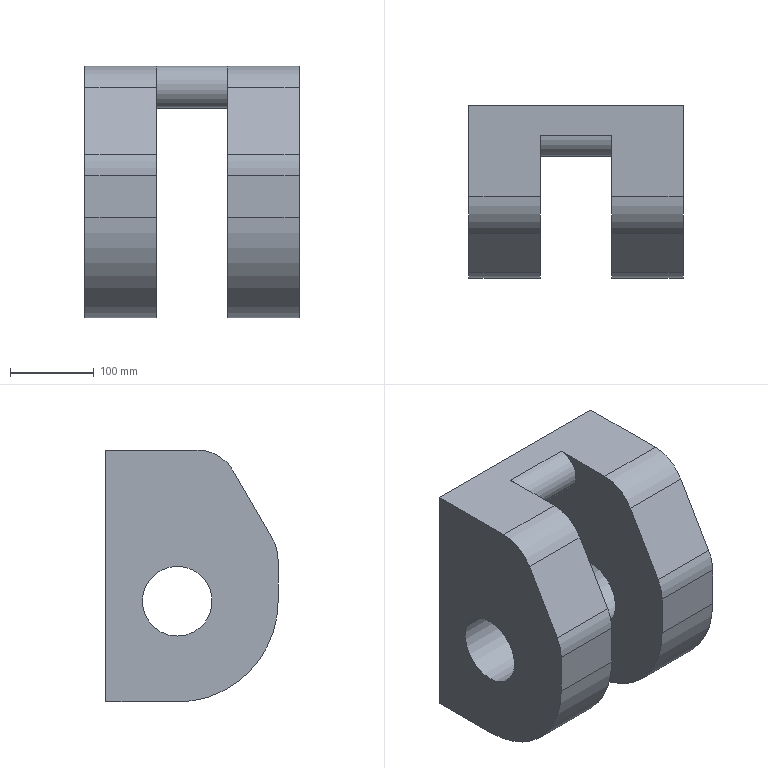Part | NX | features solid 2 | 1 solid | 22 faces | box 255 x 205 x 300 mm | volume 8542229 mm3 | plane 13 | cylinder 9 | commonest cylinder face diameters 100 x4 83 x2 240 x2 50 x1
STEP:
#1=CARTESIAN_POINT('',(-1395.,-1008.453,380.));
#2=VERTEX_POINT('',#1);
#3=CARTESIAN_POINT('',(-1395.,-935.,380.));
#4=VERTEX_POINT('',#3);
#5=CARTESIAN_POINT('',(-1395.,-1105.,380.));
#6=DIRECTION('',(0.,1.,0.));
#7=VECTOR('',#6,1000.);
#8=LINE('',#5,#7);
#9=EDGE_CURVE('',#2,#4,#8,.T.);
#10=ORIENTED_EDGE('',*,*,#9,.F.);
#11=CARTESIAN_POINT('',(-1310.,-1008.453,380.));
#12=VERTEX_POINT('',#11);
#13=CARTESIAN_POINT('',(-1310.,-1008.453,380.));
#14=DIRECTION('',(1.,0.,0.));
#15=VECTOR('',#14,1000.);
#16=LINE('',#13,#15);
#17=EDGE_CURVE('',#2,#12,#16,.T.);
#18=ORIENTED_EDGE('',*,*,#17,.T.);
#19=CARTESIAN_POINT('',(-1310.,-900.,380.));
#20=VERTEX_POINT('',#19);
#21=CARTESIAN_POINT('',(-1310.,-1105.,380.));
#22=DIRECTION('',(0.,1.,0.));
#23=VECTOR('',#22,1000.);
#24=LINE('',#21,#23);
#25=EDGE_CURVE('',#12,#20,#24,.T.);
#26=ORIENTED_EDGE('',*,*,#25,.T.);
#27=CARTESIAN_POINT('',(-1565.,-900.,380.));
#28=VERTEX_POINT('',#27);
#29=CARTESIAN_POINT('',(-1565.,-900.,380.));
#30=DIRECTION('',(1.,0.,0.));
#31=VECTOR('',#30,1000.);
#32=LINE('',#29,#31);
#33=EDGE_CURVE('',#28,#20,#32,.T.);
#34=ORIENTED_EDGE('',*,*,#33,.F.);
#35=CARTESIAN_POINT('',(-1565.,-1008.453,380.));
#36=VERTEX_POINT('',#35);
#37=CARTESIAN_POINT('',(-1565.,-1105.,380.));
#38=DIRECTION('',(0.,1.,0.));
#39=VECTOR('',#38,1000.);
#40=LINE('',#37,#39);
#41=EDGE_CURVE('',#36,#28,#40,.T.);
#42=ORIENTED_EDGE('',*,*,#41,.F.);
#43=CARTESIAN_POINT('',(-1480.,-1008.453,380.));
#44=VERTEX_POINT('',#43);
#45=CARTESIAN_POINT('',(-1480.,-1008.453,380.));
#46=DIRECTION('',(1.,0.,0.));
#47=VECTOR('',#46,1000.);
#48=LINE('',#45,#47);
#49=EDGE_CURVE('',#36,#44,#48,.T.);
#50=ORIENTED_EDGE('',*,*,#49,.T.);
#51=CARTESIAN_POINT('',(-1480.,-935.,380.));
#52=VERTEX_POINT('',#51);
#53=CARTESIAN_POINT('',(-1480.,-1105.,380.));
#54=DIRECTION('',(0.,1.,0.));
#55=VECTOR('',#54,1000.);
#56=LINE('',#53,#55);
#57=EDGE_CURVE('',#44,#52,#56,.T.);
#58=ORIENTED_EDGE('',*,*,#57,.T.);
#59=CARTESIAN_POINT('',(-1437.5,-935.,380.));
#60=DIRECTION('',(1.,0.,0.));
#61=VECTOR('',#60,1000.);
#62=LINE('',#59,#61);
#63=EDGE_CURVE('',#4,#52,#62,.F.);
#64=ORIENTED_EDGE('',*,*,#63,.F.);
#65=EDGE_LOOP('',(#10,#18,#26,#34,#42,#50,#58,#64));
#66=FACE_BOUND('',#65,.T.);
#67=CARTESIAN_POINT('',(-1565.,-1105.,380.));
#68=DIRECTION('',(0.,0.,-1.));
#69=DIRECTION('',(0.,1.,0.));
#70=AXIS2_PLACEMENT_3D('',#67,#68,#69);
#71=PLANE('',#70);
#72=ADVANCED_FACE('',(#66),#71,.F.);
#73=CARTESIAN_POINT('',(-1565.,-985.,80.));
#74=VERTEX_POINT('',#73);
#75=CARTESIAN_POINT('',(-1565.,-900.,80.));
#76=VERTEX_POINT('',#75);
#77=CARTESIAN_POINT('',(-1565.,-1105.,80.));
#78=DIRECTION('',(0.,1.,0.));
#79=VECTOR('',#78,1000.);
#80=LINE('',#77,#79);
#81=EDGE_CURVE('',#74,#76,#80,.T.);
#82=ORIENTED_EDGE('',*,*,#81,.T.);
#83=CARTESIAN_POINT('',(-1480.,-900.,80.));
#84=VERTEX_POINT('',#83);
#85=CARTESIAN_POINT('',(-1565.,-900.,80.));
#86=DIRECTION('',(1.,0.,0.));
#87=VECTOR('',#86,1000.);
#88=LINE('',#85,#87);
#89=EDGE_CURVE('',#76,#84,#88,.T.);
#90=ORIENTED_EDGE('',*,*,#89,.T.);
#91=CARTESIAN_POINT('',(-1480.,-985.,80.));
#92=VERTEX_POINT('',#91);
#93=CARTESIAN_POINT('',(-1480.,-1105.,80.));
#94=DIRECTION('',(0.,-1.,0.));
#95=VECTOR('',#94,1000.);
#96=LINE('',#93,#95);
#97=EDGE_CURVE('',#92,#84,#96,.F.);
#98=ORIENTED_EDGE('',*,*,#97,.F.);
#99=CARTESIAN_POINT('',(-1565.,-985.,80.));
#100=DIRECTION('',(-1.,0.,0.));
#101=VECTOR('',#100,1000.);
#102=LINE('',#99,#101);
#103=EDGE_CURVE('',#74,#92,#102,.F.);
#104=ORIENTED_EDGE('',*,*,#103,.F.);
#105=EDGE_LOOP('',(#82,#90,#98,#104));
#106=FACE_BOUND('',#105,.T.);
#107=CARTESIAN_POINT('',(-1565.,-1105.,80.));
#108=DIRECTION('',(0.,0.,-1.));
#109=DIRECTION('',(0.,1.,0.));
#110=AXIS2_PLACEMENT_3D('',#107,#108,#109);
#111=PLANE('',#110);
#112=ADVANCED_FACE('',(#106),#111,.T.);
#113=CARTESIAN_POINT('',(-1480.,-1105.,200.));
#114=VERTEX_POINT('',#113);
#115=CARTESIAN_POINT('',(-1480.,-1105.,249.378));
#116=VERTEX_POINT('',#115);
#117=CARTESIAN_POINT('',(-1480.,-1105.,80.));
#118=DIRECTION('',(0.,0.,1.));
#119=VECTOR('',#118,1000.);
#120=LINE('',#117,#119);
#121=EDGE_CURVE('',#114,#116,#120,.T.);
#122=ORIENTED_EDGE('',*,*,#121,.T.);
#123=CARTESIAN_POINT('',(-1565.,-1105.,249.378));
#124=VERTEX_POINT('',#123);
#125=CARTESIAN_POINT('',(-1565.,-1105.,249.378));
#126=DIRECTION('',(-1.,0.,0.));
#127=VECTOR('',#126,1000.);
#128=LINE('',#125,#127);
#129=EDGE_CURVE('',#116,#124,#128,.T.);
#130=ORIENTED_EDGE('',*,*,#129,.T.);
#131=CARTESIAN_POINT('',(-1565.,-1105.,200.));
#132=VERTEX_POINT('',#131);
#133=CARTESIAN_POINT('',(-1565.,-1105.,80.));
#134=DIRECTION('',(0.,0.,1.));
#135=VECTOR('',#134,1000.);
#136=LINE('',#133,#135);
#137=EDGE_CURVE('',#132,#124,#136,.T.);
#138=ORIENTED_EDGE('',*,*,#137,.F.);
#139=CARTESIAN_POINT('',(-1565.,-1105.,200.));
#140=DIRECTION('',(1.,0.,0.));
#141=VECTOR('',#140,1000.);
#142=LINE('',#139,#141);
#143=EDGE_CURVE('',#114,#132,#142,.F.);
#144=ORIENTED_EDGE('',*,*,#143,.F.);
#145=EDGE_LOOP('',(#122,#130,#138,#144));
#146=FACE_BOUND('',#145,.T.);
#147=CARTESIAN_POINT('',(-1565.,-1105.,80.));
#148=DIRECTION('',(0.,1.,0.));
#149=DIRECTION('',(0.,0.,1.));
#150=AXIS2_PLACEMENT_3D('',#147,#148,#149);
#151=PLANE('',#150);
#152=ADVANCED_FACE('',(#146),#151,.F.);
#153=CARTESIAN_POINT('',(-1310.,-900.,80.));
#154=VERTEX_POINT('',#153);
#155=CARTESIAN_POINT('',(-1310.,-900.,45.));
#156=DIRECTION('',(0.,0.,1.));
#157=VECTOR('',#156,1000.);
#158=LINE('',#155,#157);
#159=EDGE_CURVE('',#154,#20,#158,.T.);
#160=ORIENTED_EDGE('',*,*,#159,.F.);
#161=CARTESIAN_POINT('',(-1395.,-900.,80.));
#162=VERTEX_POINT('',#161);
#163=CARTESIAN_POINT('',(-1395.,-900.,80.));
#164=DIRECTION('',(1.,0.,0.));
#165=VECTOR('',#164,1000.);
#166=LINE('',#163,#165);
#167=EDGE_CURVE('',#162,#154,#166,.T.);
#168=ORIENTED_EDGE('',*,*,#167,.F.);
#169=CARTESIAN_POINT('',(-1395.,-900.,330.));
#170=VERTEX_POINT('',#169);
#171=CARTESIAN_POINT('',(-1395.,-900.,45.));
#172=DIRECTION('',(0.,0.,1.));
#173=VECTOR('',#172,1000.);
#174=LINE('',#171,#173);
#175=EDGE_CURVE('',#162,#170,#174,.T.);
#176=ORIENTED_EDGE('',*,*,#175,.T.);
#177=CARTESIAN_POINT('',(-1480.,-900.,330.));
#178=VERTEX_POINT('',#177);
#179=CARTESIAN_POINT('',(-1437.5,-900.,330.));
#180=DIRECTION('',(1.,0.,0.));
#181=VECTOR('',#180,1000.);
#182=LINE('',#179,#181);
#183=EDGE_CURVE('',#178,#170,#182,.T.);
#184=ORIENTED_EDGE('',*,*,#183,.F.);
#185=CARTESIAN_POINT('',(-1480.,-900.,45.));
#186=DIRECTION('',(0.,0.,1.));
#187=VECTOR('',#186,1000.);
#188=LINE('',#185,#187);
#189=EDGE_CURVE('',#84,#178,#188,.T.);
#190=ORIENTED_EDGE('',*,*,#189,.F.);
#191=ORIENTED_EDGE('',*,*,#89,.F.);
#192=CARTESIAN_POINT('',(-1565.,-900.,45.));
#193=DIRECTION('',(0.,0.,1.));
#194=VECTOR('',#193,1000.);
#195=LINE('',#192,#194);
#196=EDGE_CURVE('',#76,#28,#195,.T.);
#197=ORIENTED_EDGE('',*,*,#196,.T.);
#198=ORIENTED_EDGE('',*,*,#33,.T.);
#199=EDGE_LOOP('',(#160,#168,#176,#184,#190,#191,#197,#198));
#200=FACE_BOUND('',#199,.T.);
#201=CARTESIAN_POINT('',(-1565.,-900.,45.));
#202=DIRECTION('',(0.,1.,0.));
#203=DIRECTION('',(0.,0.,1.));
#204=AXIS2_PLACEMENT_3D('',#201,#202,#203);
#205=PLANE('',#204);
#206=ADVANCED_FACE('',(#200),#205,.T.);
#207=ORIENTED_EDGE('',*,*,#57,.F.);
#208=CARTESIAN_POINT('',(-1480.,-1051.754,355.));
#209=VERTEX_POINT('',#208);
#210=CARTESIAN_POINT('',(-1480.,-1008.453,330.));
#211=DIRECTION('',(-1.,0.,0.));
#212=DIRECTION('',(0.,0.,-1.));
#213=AXIS2_PLACEMENT_3D('',#210,#211,#212);
#214=CIRCLE('',#213,50.);
#215=EDGE_CURVE('',#44,#209,#214,.F.);
#216=ORIENTED_EDGE('',*,*,#215,.T.);
#217=CARTESIAN_POINT('',(-1480.,-1098.301,274.378));
#218=VERTEX_POINT('',#217);
#219=CARTESIAN_POINT('',(-1480.,-1174.286,142.769));
#220=DIRECTION('',(0.,0.5,0.866));
#221=VECTOR('',#220,1000.);
#222=LINE('',#219,#221);
#223=EDGE_CURVE('',#218,#209,#222,.T.);
#224=ORIENTED_EDGE('',*,*,#223,.F.);
#225=CARTESIAN_POINT('',(-1480.,-1055.,249.378));
#226=DIRECTION('',(-1.,0.,0.));
#227=DIRECTION('',(0.,0.,-1.));
#228=AXIS2_PLACEMENT_3D('',#225,#226,#227);
#229=CIRCLE('',#228,50.);
#230=EDGE_CURVE('',#218,#116,#229,.F.);
#231=ORIENTED_EDGE('',*,*,#230,.T.);
#232=ORIENTED_EDGE('',*,*,#121,.F.);
#233=CARTESIAN_POINT('',(-1480.,-985.,200.));
#234=DIRECTION('',(1.,0.,0.));
#235=DIRECTION('',(0.,0.,1.));
#236=AXIS2_PLACEMENT_3D('',#233,#234,#235);
#237=CIRCLE('',#236,120.);
#238=EDGE_CURVE('',#92,#114,#237,.F.);
#239=ORIENTED_EDGE('',*,*,#238,.F.);
#240=ORIENTED_EDGE('',*,*,#97,.T.);
#241=ORIENTED_EDGE('',*,*,#189,.T.);
#242=CARTESIAN_POINT('',(-1480.,-935.,330.));
#243=VERTEX_POINT('',#242);
#244=CARTESIAN_POINT('',(-1480.,-930.,330.));
#245=DIRECTION('',(0.,1.,0.));
#246=VECTOR('',#245,1000.);
#247=LINE('',#244,#246);
#248=EDGE_CURVE('',#243,#178,#247,.T.);
#249=ORIENTED_EDGE('',*,*,#248,.F.);
#250=CARTESIAN_POINT('',(-1480.,-935.,355.));
#251=DIRECTION('',(1.,0.,0.));
#252=DIRECTION('',(0.,0.,1.));
#253=AXIS2_PLACEMENT_3D('',#250,#251,#252);
#254=CIRCLE('',#253,25.);
#255=EDGE_CURVE('',#52,#243,#254,.T.);
#256=ORIENTED_EDGE('',*,*,#255,.F.);
#257=EDGE_LOOP('',(#207,#216,#224,#231,#232,#239,#240,#241,#249,#256));
#258=FACE_BOUND('',#257,.T.);
#259=CARTESIAN_POINT('',(-1480.,-985.,241.5));
#260=VERTEX_POINT('',#259);
#261=CARTESIAN_POINT('',(-1480.,-985.,200.));
#262=DIRECTION('',(1.,0.,0.));
#263=DIRECTION('',(0.,0.,1.));
#264=AXIS2_PLACEMENT_3D('',#261,#262,#263);
#265=CIRCLE('',#264,41.5);
#266=EDGE_CURVE('',#260,#260,#265,.T.);
#267=ORIENTED_EDGE('',*,*,#266,.F.);
#268=EDGE_LOOP('',(#267));
#269=FACE_BOUND('',#268,.T.);
#270=CARTESIAN_POINT('',(-1480.,-1105.,45.));
#271=DIRECTION('',(-1.,0.,0.));
#272=DIRECTION('',(0.,0.,1.));
#273=AXIS2_PLACEMENT_3D('',#270,#271,#272);
#274=PLANE('',#273);
#275=ADVANCED_FACE('',(#258,#269),#274,.F.);
#276=CARTESIAN_POINT('',(-1565.,-1098.301,274.378));
#277=VERTEX_POINT('',#276);
#278=CARTESIAN_POINT('',(-1565.,-1051.754,355.));
#279=VERTEX_POINT('',#278);
#280=CARTESIAN_POINT('',(-1565.,-1174.286,142.769));
#281=DIRECTION('',(0.,0.5,0.866));
#282=VECTOR('',#281,1000.);
#283=LINE('',#280,#282);
#284=EDGE_CURVE('',#277,#279,#283,.T.);
#285=ORIENTED_EDGE('',*,*,#284,.T.);
#286=CARTESIAN_POINT('',(-1565.,-1008.453,330.));
#287=DIRECTION('',(-1.,0.,0.));
#288=DIRECTION('',(0.,0.,-1.));
#289=AXIS2_PLACEMENT_3D('',#286,#287,#288);
#290=CIRCLE('',#289,50.);
#291=EDGE_CURVE('',#279,#36,#290,.T.);
#292=ORIENTED_EDGE('',*,*,#291,.T.);
#293=ORIENTED_EDGE('',*,*,#41,.T.);
#294=ORIENTED_EDGE('',*,*,#196,.F.);
#295=ORIENTED_EDGE('',*,*,#81,.F.);
#296=CARTESIAN_POINT('',(-1565.,-985.,200.));
#297=DIRECTION('',(1.,0.,0.));
#298=DIRECTION('',(0.,0.,1.));
#299=AXIS2_PLACEMENT_3D('',#296,#297,#298);
#300=CIRCLE('',#299,120.);
#301=EDGE_CURVE('',#132,#74,#300,.T.);
#302=ORIENTED_EDGE('',*,*,#301,.F.);
#303=ORIENTED_EDGE('',*,*,#137,.T.);
#304=CARTESIAN_POINT('',(-1565.,-1055.,249.378));
#305=DIRECTION('',(-1.,0.,0.));
#306=DIRECTION('',(0.,0.,-1.));
#307=AXIS2_PLACEMENT_3D('',#304,#305,#306);
#308=CIRCLE('',#307,50.);
#309=EDGE_CURVE('',#124,#277,#308,.T.);
#310=ORIENTED_EDGE('',*,*,#309,.T.);
#311=EDGE_LOOP('',(#285,#292,#293,#294,#295,#302,#303,#310));
#312=FACE_BOUND('',#311,.T.);
#313=CARTESIAN_POINT('',(-1565.,-985.,158.5));
#314=VERTEX_POINT('',#313);
#315=CARTESIAN_POINT('',(-1565.,-985.,200.));
#316=DIRECTION('',(-1.,0.,0.));
#317=DIRECTION('',(0.,0.,-1.));
#318=AXIS2_PLACEMENT_3D('',#315,#316,#317);
#319=CIRCLE('',#318,41.5);
#320=EDGE_CURVE('',#314,#314,#319,.T.);
#321=ORIENTED_EDGE('',*,*,#320,.F.);
#322=EDGE_LOOP('',(#321));
#323=FACE_BOUND('',#322,.T.);
#324=CARTESIAN_POINT('',(-1565.,-1105.,45.));
#325=DIRECTION('',(-1.,0.,0.));
#326=DIRECTION('',(0.,0.,1.));
#327=AXIS2_PLACEMENT_3D('',#324,#325,#326);
#328=PLANE('',#327);
#329=ADVANCED_FACE('',(#312,#323),#328,.T.);
#330=ORIENTED_EDGE('',*,*,#301,.T.);
#331=ORIENTED_EDGE('',*,*,#103,.T.);
#332=ORIENTED_EDGE('',*,*,#238,.T.);
#333=ORIENTED_EDGE('',*,*,#143,.T.);
#334=EDGE_LOOP('',(#330,#331,#332,#333));
#335=FACE_BOUND('',#334,.T.);
#336=CARTESIAN_POINT('',(-1565.,-985.,200.));
#337=DIRECTION('',(-1.,0.,0.));
#338=DIRECTION('',(0.,0.,1.));
#339=AXIS2_PLACEMENT_3D('',#336,#337,#338);
#340=CYLINDRICAL_SURFACE('',#339,120.);
#341=ADVANCED_FACE('',(#335),#340,.T.);
#342=ORIENTED_EDGE('',*,*,#320,.T.);
#343=EDGE_LOOP('',(#342));
#344=FACE_BOUND('',#343,.T.);
#345=ORIENTED_EDGE('',*,*,#266,.T.);
#346=EDGE_LOOP('',(#345));
#347=FACE_BOUND('',#346,.T.);
#348=CARTESIAN_POINT('',(-1565.,-985.,200.));
#349=DIRECTION('',(1.,0.,0.));
#350=DIRECTION('',(0.,0.,-1.));
#351=AXIS2_PLACEMENT_3D('',#348,#349,#350);
#352=CYLINDRICAL_SURFACE('',#351,41.5);
#353=ADVANCED_FACE('',(#344,#347),#352,.F.);
#354=ORIENTED_EDGE('',*,*,#248,.T.);
#355=ORIENTED_EDGE('',*,*,#183,.T.);
#356=CARTESIAN_POINT('',(-1395.,-935.,330.));
#357=VERTEX_POINT('',#356);
#358=CARTESIAN_POINT('',(-1395.,-930.,330.));
#359=DIRECTION('',(0.,-1.,0.));
#360=VECTOR('',#359,1000.);
#361=LINE('',#358,#360);
#362=EDGE_CURVE('',#170,#357,#361,.T.);
#363=ORIENTED_EDGE('',*,*,#362,.T.);
#364=CARTESIAN_POINT('',(-1437.5,-935.,330.));
#365=DIRECTION('',(-1.,0.,0.));
#366=VECTOR('',#365,1000.);
#367=LINE('',#364,#366);
#368=EDGE_CURVE('',#243,#357,#367,.F.);
#369=ORIENTED_EDGE('',*,*,#368,.F.);
#370=EDGE_LOOP('',(#354,#355,#363,#369));
#371=FACE_BOUND('',#370,.T.);
#372=CARTESIAN_POINT('',(-1437.5,-930.,330.));
#373=DIRECTION('',(0.,0.,-1.));
#374=DIRECTION('',(0.,-1.,0.));
#375=AXIS2_PLACEMENT_3D('',#372,#373,#374);
#376=PLANE('',#375);
#377=ADVANCED_FACE('',(#371),#376,.T.);
#378=ORIENTED_EDGE('',*,*,#368,.T.);
#379=CARTESIAN_POINT('',(-1395.,-935.,355.));
#380=DIRECTION('',(-1.,0.,0.));
#381=DIRECTION('',(0.,0.,-1.));
#382=AXIS2_PLACEMENT_3D('',#379,#380,#381);
#383=CIRCLE('',#382,25.);
#384=EDGE_CURVE('',#357,#4,#383,.T.);
#385=ORIENTED_EDGE('',*,*,#384,.T.);
#386=ORIENTED_EDGE('',*,*,#63,.T.);
#387=ORIENTED_EDGE('',*,*,#255,.T.);
#388=EDGE_LOOP('',(#378,#385,#386,#387));
#389=FACE_BOUND('',#388,.T.);
#390=CARTESIAN_POINT('',(-1437.5,-935.,355.));
#391=DIRECTION('',(-1.,0.,0.));
#392=DIRECTION('',(0.,0.,1.));
#393=AXIS2_PLACEMENT_3D('',#390,#391,#392);
#394=CYLINDRICAL_SURFACE('',#393,25.);
#395=ADVANCED_FACE('',(#389),#394,.T.);
#396=CARTESIAN_POINT('',(-1395.,-985.,80.));
#397=VERTEX_POINT('',#396);
#398=CARTESIAN_POINT('',(-1395.,-1105.,80.));
#399=DIRECTION('',(0.,1.,0.));
#400=VECTOR('',#399,1000.);
#401=LINE('',#398,#400);
#402=EDGE_CURVE('',#397,#162,#401,.T.);
#403=ORIENTED_EDGE('',*,*,#402,.T.);
#404=ORIENTED_EDGE('',*,*,#167,.T.);
#405=CARTESIAN_POINT('',(-1310.,-985.,80.));
#406=VERTEX_POINT('',#405);
#407=CARTESIAN_POINT('',(-1310.,-1105.,80.));
#408=DIRECTION('',(0.,-1.,0.));
#409=VECTOR('',#408,1000.);
#410=LINE('',#407,#409);
#411=EDGE_CURVE('',#406,#154,#410,.F.);
#412=ORIENTED_EDGE('',*,*,#411,.F.);
#413=CARTESIAN_POINT('',(-1395.,-985.,80.));
#414=DIRECTION('',(-1.,0.,0.));
#415=VECTOR('',#414,1000.);
#416=LINE('',#413,#415);
#417=EDGE_CURVE('',#397,#406,#416,.F.);
#418=ORIENTED_EDGE('',*,*,#417,.F.);
#419=EDGE_LOOP('',(#403,#404,#412,#418));
#420=FACE_BOUND('',#419,.T.);
#421=CARTESIAN_POINT('',(-1395.,-1105.,80.));
#422=DIRECTION('',(0.,0.,-1.));
#423=DIRECTION('',(0.,1.,0.));
#424=AXIS2_PLACEMENT_3D('',#421,#422,#423);
#425=PLANE('',#424);
#426=ADVANCED_FACE('',(#420),#425,.T.);
#427=CARTESIAN_POINT('',(-1310.,-1105.,200.));
#428=VERTEX_POINT('',#427);
#429=CARTESIAN_POINT('',(-1310.,-1105.,249.378));
#430=VERTEX_POINT('',#429);
#431=CARTESIAN_POINT('',(-1310.,-1105.,80.));
#432=DIRECTION('',(0.,0.,1.));
#433=VECTOR('',#432,1000.);
#434=LINE('',#431,#433);
#435=EDGE_CURVE('',#428,#430,#434,.T.);
#436=ORIENTED_EDGE('',*,*,#435,.T.);
#437=CARTESIAN_POINT('',(-1395.,-1105.,249.378));
#438=VERTEX_POINT('',#437);
#439=CARTESIAN_POINT('',(-1395.,-1105.,249.378));
#440=DIRECTION('',(-1.,0.,0.));
#441=VECTOR('',#440,1000.);
#442=LINE('',#439,#441);
#443=EDGE_CURVE('',#430,#438,#442,.T.);
#444=ORIENTED_EDGE('',*,*,#443,.T.);
#445=CARTESIAN_POINT('',(-1395.,-1105.,200.));
#446=VERTEX_POINT('',#445);
#447=CARTESIAN_POINT('',(-1395.,-1105.,80.));
#448=DIRECTION('',(0.,0.,1.));
#449=VECTOR('',#448,1000.);
#450=LINE('',#447,#449);
#451=EDGE_CURVE('',#446,#438,#450,.T.);
#452=ORIENTED_EDGE('',*,*,#451,.F.);
#453=CARTESIAN_POINT('',(-1395.,-1105.,200.));
#454=DIRECTION('',(1.,0.,0.));
#455=VECTOR('',#454,1000.);
#456=LINE('',#453,#455);
#457=EDGE_CURVE('',#428,#446,#456,.F.);
#458=ORIENTED_EDGE('',*,*,#457,.F.);
#459=EDGE_LOOP('',(#436,#444,#452,#458));
#460=FACE_BOUND('',#459,.T.);
#461=CARTESIAN_POINT('',(-1395.,-1105.,80.));
#462=DIRECTION('',(0.,1.,0.));
#463=DIRECTION('',(0.,0.,1.));
#464=AXIS2_PLACEMENT_3D('',#461,#462,#463);
#465=PLANE('',#464);
#466=ADVANCED_FACE('',(#460),#465,.F.);
#467=ORIENTED_EDGE('',*,*,#25,.F.);
#468=CARTESIAN_POINT('',(-1310.,-1051.754,355.));
#469=VERTEX_POINT('',#468);
#470=CARTESIAN_POINT('',(-1310.,-1008.453,330.));
#471=DIRECTION('',(-1.,0.,0.));
#472=DIRECTION('',(0.,0.,-1.));
#473=AXIS2_PLACEMENT_3D('',#470,#471,#472);
#474=CIRCLE('',#473,50.);
#475=EDGE_CURVE('',#12,#469,#474,.F.);
#476=ORIENTED_EDGE('',*,*,#475,.T.);
#477=CARTESIAN_POINT('',(-1310.,-1098.301,274.378));
#478=VERTEX_POINT('',#477);
#479=CARTESIAN_POINT('',(-1310.,-1174.286,142.769));
#480=DIRECTION('',(0.,0.5,0.866));
#481=VECTOR('',#480,1000.);
#482=LINE('',#479,#481);
#483=EDGE_CURVE('',#478,#469,#482,.T.);
#484=ORIENTED_EDGE('',*,*,#483,.F.);
#485=CARTESIAN_POINT('',(-1310.,-1055.,249.378));
#486=DIRECTION('',(-1.,0.,0.));
#487=DIRECTION('',(0.,0.,-1.));
#488=AXIS2_PLACEMENT_3D('',#485,#486,#487);
#489=CIRCLE('',#488,50.);
#490=EDGE_CURVE('',#478,#430,#489,.F.);
#491=ORIENTED_EDGE('',*,*,#490,.T.);
#492=ORIENTED_EDGE('',*,*,#435,.F.);
#493=CARTESIAN_POINT('',(-1310.,-985.,200.));
#494=DIRECTION('',(1.,0.,0.));
#495=DIRECTION('',(0.,0.,1.));
#496=AXIS2_PLACEMENT_3D('',#493,#494,#495);
#497=CIRCLE('',#496,120.);
#498=EDGE_CURVE('',#406,#428,#497,.F.);
#499=ORIENTED_EDGE('',*,*,#498,.F.);
#500=ORIENTED_EDGE('',*,*,#411,.T.);
#501=ORIENTED_EDGE('',*,*,#159,.T.);
#502=EDGE_LOOP('',(#467,#476,#484,#491,#492,#499,#500,#501));
#503=FACE_BOUND('',#502,.T.);
#504=CARTESIAN_POINT('',(-1310.,-985.,241.5));
#505=VERTEX_POINT('',#504);
#506=CARTESIAN_POINT('',(-1310.,-985.,200.));
#507=DIRECTION('',(1.,0.,0.));
#508=DIRECTION('',(0.,0.,1.));
#509=AXIS2_PLACEMENT_3D('',#506,#507,#508);
#510=CIRCLE('',#509,41.5);
#511=EDGE_CURVE('',#505,#505,#510,.T.);
#512=ORIENTED_EDGE('',*,*,#511,.F.);
#513=EDGE_LOOP('',(#512));
#514=FACE_BOUND('',#513,.T.);
#515=CARTESIAN_POINT('',(-1310.,-1105.,45.));
#516=DIRECTION('',(-1.,0.,0.));
#517=DIRECTION('',(0.,0.,1.));
#518=AXIS2_PLACEMENT_3D('',#515,#516,#517);
#519=PLANE('',#518);
#520=ADVANCED_FACE('',(#503,#514),#519,.F.);
#521=CARTESIAN_POINT('',(-1395.,-1098.301,274.378));
#522=VERTEX_POINT('',#521);
#523=CARTESIAN_POINT('',(-1395.,-1051.754,355.));
#524=VERTEX_POINT('',#523);
#525=CARTESIAN_POINT('',(-1395.,-1174.286,142.769));
#526=DIRECTION('',(0.,0.5,0.866));
#527=VECTOR('',#526,1000.);
#528=LINE('',#525,#527);
#529=EDGE_CURVE('',#522,#524,#528,.T.);
#530=ORIENTED_EDGE('',*,*,#529,.T.);
#531=CARTESIAN_POINT('',(-1395.,-1008.453,330.));
#532=DIRECTION('',(-1.,0.,0.));
#533=DIRECTION('',(0.,0.,-1.));
#534=AXIS2_PLACEMENT_3D('',#531,#532,#533);
#535=CIRCLE('',#534,50.);
#536=EDGE_CURVE('',#524,#2,#535,.T.);
#537=ORIENTED_EDGE('',*,*,#536,.T.);
#538=ORIENTED_EDGE('',*,*,#9,.T.);
#539=ORIENTED_EDGE('',*,*,#384,.F.);
#540=ORIENTED_EDGE('',*,*,#362,.F.);
#541=ORIENTED_EDGE('',*,*,#175,.F.);
#542=ORIENTED_EDGE('',*,*,#402,.F.);
#543=CARTESIAN_POINT('',(-1395.,-985.,200.));
#544=DIRECTION('',(1.,0.,0.));
#545=DIRECTION('',(0.,0.,1.));
#546=AXIS2_PLACEMENT_3D('',#543,#544,#545);
#547=CIRCLE('',#546,120.);
#548=EDGE_CURVE('',#446,#397,#547,.T.);
#549=ORIENTED_EDGE('',*,*,#548,.F.);
#550=ORIENTED_EDGE('',*,*,#451,.T.);
#551=CARTESIAN_POINT('',(-1395.,-1055.,249.378));
#552=DIRECTION('',(-1.,0.,0.));
#553=DIRECTION('',(0.,0.,-1.));
#554=AXIS2_PLACEMENT_3D('',#551,#552,#553);
#555=CIRCLE('',#554,50.);
#556=EDGE_CURVE('',#438,#522,#555,.T.);
#557=ORIENTED_EDGE('',*,*,#556,.T.);
#558=EDGE_LOOP('',(#530,#537,#538,#539,#540,#541,#542,#549,#550,#557));
#559=FACE_BOUND('',#558,.T.);
#560=CARTESIAN_POINT('',(-1395.,-985.,158.5));
#561=VERTEX_POINT('',#560);
#562=CARTESIAN_POINT('',(-1395.,-985.,200.));
#563=DIRECTION('',(-1.,0.,0.));
#564=DIRECTION('',(0.,0.,-1.));
#565=AXIS2_PLACEMENT_3D('',#562,#563,#564);
#566=CIRCLE('',#565,41.5);
#567=EDGE_CURVE('',#561,#561,#566,.T.);
#568=ORIENTED_EDGE('',*,*,#567,.F.);
#569=EDGE_LOOP('',(#568));
#570=FACE_BOUND('',#569,.T.);
#571=CARTESIAN_POINT('',(-1395.,-1105.,45.));
#572=DIRECTION('',(-1.,0.,0.));
#573=DIRECTION('',(0.,0.,1.));
#574=AXIS2_PLACEMENT_3D('',#571,#572,#573);
#575=PLANE('',#574);
#576=ADVANCED_FACE('',(#559,#570),#575,.T.);
#577=ORIENTED_EDGE('',*,*,#548,.T.);
#578=ORIENTED_EDGE('',*,*,#417,.T.);
#579=ORIENTED_EDGE('',*,*,#498,.T.);
#580=ORIENTED_EDGE('',*,*,#457,.T.);
#581=EDGE_LOOP('',(#577,#578,#579,#580));
#582=FACE_BOUND('',#581,.T.);
#583=CARTESIAN_POINT('',(-1395.,-985.,200.));
#584=DIRECTION('',(-1.,0.,0.));
#585=DIRECTION('',(0.,0.,1.));
#586=AXIS2_PLACEMENT_3D('',#583,#584,#585);
#587=CYLINDRICAL_SURFACE('',#586,120.);
#588=ADVANCED_FACE('',(#582),#587,.T.);
#589=ORIENTED_EDGE('',*,*,#567,.T.);
#590=EDGE_LOOP('',(#589));
#591=FACE_BOUND('',#590,.T.);
#592=ORIENTED_EDGE('',*,*,#511,.T.);
#593=EDGE_LOOP('',(#592));
#594=FACE_BOUND('',#593,.T.);
#595=CARTESIAN_POINT('',(-1395.,-985.,200.));
#596=DIRECTION('',(1.,0.,0.));
#597=DIRECTION('',(0.,0.,-1.));
#598=AXIS2_PLACEMENT_3D('',#595,#596,#597);
#599=CYLINDRICAL_SURFACE('',#598,41.5);
#600=ADVANCED_FACE('',(#591,#594),#599,.F.);
#601=ORIENTED_EDGE('',*,*,#483,.T.);
#602=CARTESIAN_POINT('',(-1395.,-1051.754,355.));
#603=DIRECTION('',(-1.,0.,0.));
#604=VECTOR('',#603,1000.);
#605=LINE('',#602,#604);
#606=EDGE_CURVE('',#469,#524,#605,.T.);
#607=ORIENTED_EDGE('',*,*,#606,.T.);
#608=ORIENTED_EDGE('',*,*,#529,.F.);
#609=CARTESIAN_POINT('',(-1310.,-1098.301,274.378));
#610=DIRECTION('',(1.,0.,0.));
#611=VECTOR('',#610,1000.);
#612=LINE('',#609,#611);
#613=EDGE_CURVE('',#522,#478,#612,.T.);
#614=ORIENTED_EDGE('',*,*,#613,.T.);
#615=EDGE_LOOP('',(#601,#607,#608,#614));
#616=FACE_BOUND('',#615,.T.);
#617=CARTESIAN_POINT('',(-1565.,-1048.868,360.));
#618=DIRECTION('',(0.,0.866,-0.5));
#619=DIRECTION('',(0.,-0.5,-0.866));
#620=AXIS2_PLACEMENT_3D('',#617,#618,#619);
#621=PLANE('',#620);
#622=ADVANCED_FACE('',(#616),#621,.F.);
#623=ORIENTED_EDGE('',*,*,#223,.T.);
#624=CARTESIAN_POINT('',(-1565.,-1051.754,355.));
#625=DIRECTION('',(-1.,0.,0.));
#626=VECTOR('',#625,1000.);
#627=LINE('',#624,#626);
#628=EDGE_CURVE('',#209,#279,#627,.T.);
#629=ORIENTED_EDGE('',*,*,#628,.T.);
#630=ORIENTED_EDGE('',*,*,#284,.F.);
#631=CARTESIAN_POINT('',(-1480.,-1098.301,274.378));
#632=DIRECTION('',(1.,0.,0.));
#633=VECTOR('',#632,1000.);
#634=LINE('',#631,#633);
#635=EDGE_CURVE('',#277,#218,#634,.T.);
#636=ORIENTED_EDGE('',*,*,#635,.T.);
#637=EDGE_LOOP('',(#623,#629,#630,#636));
#638=FACE_BOUND('',#637,.T.);
#639=CARTESIAN_POINT('',(-1565.,-1048.868,360.));
#640=DIRECTION('',(0.,0.866,-0.5));
#641=DIRECTION('',(0.,-0.5,-0.866));
#642=AXIS2_PLACEMENT_3D('',#639,#640,#641);
#643=PLANE('',#642);
#644=ADVANCED_FACE('',(#638),#643,.F.);
#645=ORIENTED_EDGE('',*,*,#536,.F.);
#646=ORIENTED_EDGE('',*,*,#606,.F.);
#647=ORIENTED_EDGE('',*,*,#475,.F.);
#648=ORIENTED_EDGE('',*,*,#17,.F.);
#649=EDGE_LOOP('',(#645,#646,#647,#648));
#650=FACE_BOUND('',#649,.T.);
#651=CARTESIAN_POINT('',(-1565.,-1008.453,330.));
#652=DIRECTION('',(1.,0.,0.));
#653=DIRECTION('',(0.,1.,0.));
#654=AXIS2_PLACEMENT_3D('',#651,#652,#653);
#655=CYLINDRICAL_SURFACE('',#654,50.);
#656=ADVANCED_FACE('',(#650),#655,.T.);
#657=ORIENTED_EDGE('',*,*,#291,.F.);
#658=ORIENTED_EDGE('',*,*,#628,.F.);
#659=ORIENTED_EDGE('',*,*,#215,.F.);
#660=ORIENTED_EDGE('',*,*,#49,.F.);
#661=EDGE_LOOP('',(#657,#658,#659,#660));
#662=FACE_BOUND('',#661,.T.);
#663=CARTESIAN_POINT('',(-1565.,-1008.453,330.));
#664=DIRECTION('',(1.,0.,0.));
#665=DIRECTION('',(0.,1.,0.));
#666=AXIS2_PLACEMENT_3D('',#663,#664,#665);
#667=CYLINDRICAL_SURFACE('',#666,50.);
#668=ADVANCED_FACE('',(#662),#667,.T.);
#669=ORIENTED_EDGE('',*,*,#490,.F.);
#670=ORIENTED_EDGE('',*,*,#613,.F.);
#671=ORIENTED_EDGE('',*,*,#556,.F.);
#672=ORIENTED_EDGE('',*,*,#443,.F.);
#673=EDGE_LOOP('',(#669,#670,#671,#672));
#674=FACE_BOUND('',#673,.T.);
#675=CARTESIAN_POINT('',(-1395.,-1055.,249.378));
#676=DIRECTION('',(-1.,0.,0.));
#677=DIRECTION('',(0.,0.,-1.));
#678=AXIS2_PLACEMENT_3D('',#675,#676,#677);
#679=CYLINDRICAL_SURFACE('',#678,50.);
#680=ADVANCED_FACE('',(#674),#679,.T.);
#681=ORIENTED_EDGE('',*,*,#230,.F.);
#682=ORIENTED_EDGE('',*,*,#635,.F.);
#683=ORIENTED_EDGE('',*,*,#309,.F.);
#684=ORIENTED_EDGE('',*,*,#129,.F.);
#685=EDGE_LOOP('',(#681,#682,#683,#684));
#686=FACE_BOUND('',#685,.T.);
#687=CARTESIAN_POINT('',(-1565.,-1055.,249.378));
#688=DIRECTION('',(-1.,0.,0.));
#689=DIRECTION('',(0.,0.,-1.));
#690=AXIS2_PLACEMENT_3D('',#687,#688,#689);
#691=CYLINDRICAL_SURFACE('',#690,50.);
#692=ADVANCED_FACE('',(#686),#691,.T.);
#693=CLOSED_SHELL('',(#72,#112,#152,#206,#275,#329,#341,#353,#377,#395,#426,#466,#520,#576,#588,#600,#622,#644,#656,#668,#680,#692));
#694=MANIFOLD_SOLID_BREP('',#693);
#695=(LENGTH_UNIT()NAMED_UNIT(*)SI_UNIT(.MILLI.,.METRE.));
#696=UNCERTAINTY_MEASURE_WITH_UNIT(LENGTH_MEASURE(0.00001),#695,'','');
#697=(NAMED_UNIT(*)PLANE_ANGLE_UNIT()SI_UNIT($,.RADIAN.));
#698=(NAMED_UNIT(*)SI_UNIT($,.STERADIAN.)SOLID_ANGLE_UNIT());
#699=(GEOMETRIC_REPRESENTATION_CONTEXT(3)GLOBAL_UNCERTAINTY_ASSIGNED_CONTEXT((#696))GLOBAL_UNIT_ASSIGNED_CONTEXT((#695,#697,#698))REPRESENTATION_CONTEXT('',''));
#700=ADVANCED_BREP_SHAPE_REPRESENTATION('',(#694),#699);